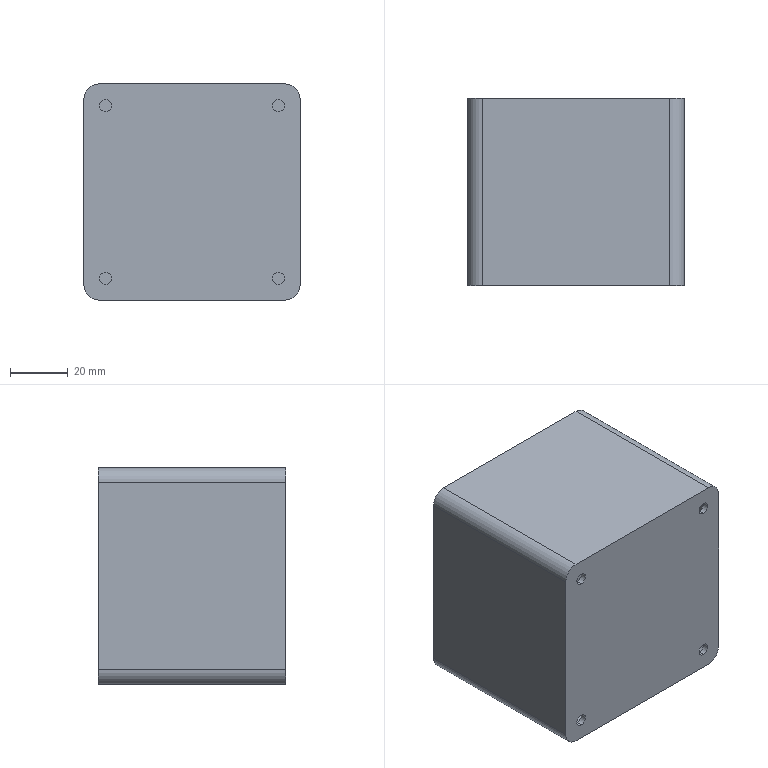Part | STEP file | Guide wheel mechanism revised.sldasm-Part-334 | 1 solid | 30 faces | box 75 x 65 x 75 mm | volume 65636 mm3 | cylinder 18 | plane 12 | commonest cylinder face diameters 4.2 x8 6 x4 10 x4 22 x2
STEP:
#1=CARTESIAN_POINT('',(30.,-30.5,32.1));
#2=VERTEX_POINT('',#1);
#3=CARTESIAN_POINT('',(30.,-30.5,27.9));
#4=VERTEX_POINT('',#3);
#5=CARTESIAN_POINT('',(30.,-30.5,30.));
#6=DIRECTION('',(0.,-1.,0.));
#7=DIRECTION('',(0.,0.,-1.));
#8=AXIS2_PLACEMENT_3D('',#5,#6,#7);
#9=CIRCLE('',#8,2.1);
#10=EDGE_CURVE('',#2,#4,#9,.T.);
#11=ORIENTED_EDGE('',*,*,#10,.F.);
#12=CARTESIAN_POINT('',(30.,-32.5,32.1));
#13=VERTEX_POINT('',#12);
#14=CARTESIAN_POINT('',(30.,-27.5,32.1));
#15=DIRECTION('',(0.,-1.,0.));
#16=VECTOR('',#15,1000.);
#17=LINE('',#14,#16);
#18=EDGE_CURVE('',#2,#13,#17,.T.);
#19=ORIENTED_EDGE('',*,*,#18,.T.);
#20=CARTESIAN_POINT('',(30.,-32.5,27.9));
#21=VERTEX_POINT('',#20);
#22=CARTESIAN_POINT('',(30.,-32.5,30.));
#23=DIRECTION('',(0.,-1.,0.));
#24=DIRECTION('',(0.,0.,1.));
#25=AXIS2_PLACEMENT_3D('',#22,#23,#24);
#26=CIRCLE('',#25,2.1);
#27=EDGE_CURVE('',#13,#21,#26,.T.);
#28=ORIENTED_EDGE('',*,*,#27,.T.);
#29=CARTESIAN_POINT('',(30.,-27.5,27.9));
#30=DIRECTION('',(0.,-1.,0.));
#31=VECTOR('',#30,1000.);
#32=LINE('',#29,#31);
#33=EDGE_CURVE('',#4,#21,#32,.T.);
#34=ORIENTED_EDGE('',*,*,#33,.F.);
#35=EDGE_LOOP('',(#11,#19,#28,#34));
#36=FACE_OUTER_BOUND('',#35,.T.);
#37=CARTESIAN_POINT('',(30.,-27.5,30.));
#38=DIRECTION('',(0.,-1.,0.));
#39=DIRECTION('',(0.,0.,-1.));
#40=AXIS2_PLACEMENT_3D('',#37,#38,#39);
#41=CYLINDRICAL_SURFACE('',#40,2.1);
#42=ADVANCED_FACE('',(#36),#41,.F.);
#43=CARTESIAN_POINT('',(30.,-30.5,-27.9));
#44=VERTEX_POINT('',#43);
#45=CARTESIAN_POINT('',(30.,-30.5,-32.1));
#46=VERTEX_POINT('',#45);
#47=CARTESIAN_POINT('',(30.,-30.5,-30.));
#48=DIRECTION('',(0.,-1.,0.));
#49=DIRECTION('',(0.,0.,-1.));
#50=AXIS2_PLACEMENT_3D('',#47,#48,#49);
#51=CIRCLE('',#50,2.1);
#52=EDGE_CURVE('',#44,#46,#51,.T.);
#53=ORIENTED_EDGE('',*,*,#52,.F.);
#54=CARTESIAN_POINT('',(30.,-32.5,-27.9));
#55=VERTEX_POINT('',#54);
#56=CARTESIAN_POINT('',(30.,-27.5,-27.9));
#57=DIRECTION('',(0.,-1.,0.));
#58=VECTOR('',#57,1000.);
#59=LINE('',#56,#58);
#60=EDGE_CURVE('',#44,#55,#59,.T.);
#61=ORIENTED_EDGE('',*,*,#60,.T.);
#62=CARTESIAN_POINT('',(30.,-32.5,-32.1));
#63=VERTEX_POINT('',#62);
#64=CARTESIAN_POINT('',(30.,-32.5,-30.));
#65=DIRECTION('',(0.,-1.,0.));
#66=DIRECTION('',(0.,0.,-1.));
#67=AXIS2_PLACEMENT_3D('',#64,#65,#66);
#68=CIRCLE('',#67,2.1);
#69=EDGE_CURVE('',#55,#63,#68,.T.);
#70=ORIENTED_EDGE('',*,*,#69,.T.);
#71=CARTESIAN_POINT('',(30.,-27.5,-32.1));
#72=DIRECTION('',(0.,-1.,0.));
#73=VECTOR('',#72,1000.);
#74=LINE('',#71,#73);
#75=EDGE_CURVE('',#46,#63,#74,.T.);
#76=ORIENTED_EDGE('',*,*,#75,.F.);
#77=EDGE_LOOP('',(#53,#61,#70,#76));
#78=FACE_OUTER_BOUND('',#77,.T.);
#79=CARTESIAN_POINT('',(30.,-27.5,-30.));
#80=DIRECTION('',(0.,-1.,0.));
#81=DIRECTION('',(0.,0.,-1.));
#82=AXIS2_PLACEMENT_3D('',#79,#80,#81);
#83=CYLINDRICAL_SURFACE('',#82,2.1);
#84=ADVANCED_FACE('',(#78),#83,.F.);
#85=CARTESIAN_POINT('',(-30.,-30.5,-27.9));
#86=VERTEX_POINT('',#85);
#87=CARTESIAN_POINT('',(-30.,-30.5,-32.1));
#88=VERTEX_POINT('',#87);
#89=CARTESIAN_POINT('',(-30.,-30.5,-30.));
#90=DIRECTION('',(0.,-1.,0.));
#91=DIRECTION('',(0.,0.,-1.));
#92=AXIS2_PLACEMENT_3D('',#89,#90,#91);
#93=CIRCLE('',#92,2.1);
#94=EDGE_CURVE('',#86,#88,#93,.T.);
#95=ORIENTED_EDGE('',*,*,#94,.F.);
#96=CARTESIAN_POINT('',(-30.,-32.5,-27.9));
#97=VERTEX_POINT('',#96);
#98=CARTESIAN_POINT('',(-30.,-27.5,-27.9));
#99=DIRECTION('',(0.,-1.,0.));
#100=VECTOR('',#99,1000.);
#101=LINE('',#98,#100);
#102=EDGE_CURVE('',#86,#97,#101,.T.);
#103=ORIENTED_EDGE('',*,*,#102,.T.);
#104=CARTESIAN_POINT('',(-30.,-32.5,-32.1));
#105=VERTEX_POINT('',#104);
#106=CARTESIAN_POINT('',(-30.,-32.5,-30.));
#107=DIRECTION('',(0.,-1.,0.));
#108=DIRECTION('',(0.,0.,1.));
#109=AXIS2_PLACEMENT_3D('',#106,#107,#108);
#110=CIRCLE('',#109,2.1);
#111=EDGE_CURVE('',#97,#105,#110,.T.);
#112=ORIENTED_EDGE('',*,*,#111,.T.);
#113=CARTESIAN_POINT('',(-30.,-27.5,-32.1));
#114=DIRECTION('',(0.,-1.,0.));
#115=VECTOR('',#114,1000.);
#116=LINE('',#113,#115);
#117=EDGE_CURVE('',#88,#105,#116,.T.);
#118=ORIENTED_EDGE('',*,*,#117,.F.);
#119=EDGE_LOOP('',(#95,#103,#112,#118));
#120=FACE_OUTER_BOUND('',#119,.T.);
#121=CARTESIAN_POINT('',(-30.,-27.5,-30.));
#122=DIRECTION('',(0.,-1.,0.));
#123=DIRECTION('',(0.,0.,-1.));
#124=AXIS2_PLACEMENT_3D('',#121,#122,#123);
#125=CYLINDRICAL_SURFACE('',#124,2.1);
#126=ADVANCED_FACE('',(#120),#125,.F.);
#127=CARTESIAN_POINT('',(-30.,-30.5,32.1));
#128=VERTEX_POINT('',#127);
#129=CARTESIAN_POINT('',(-30.,-30.5,27.9));
#130=VERTEX_POINT('',#129);
#131=CARTESIAN_POINT('',(-30.,-30.5,30.));
#132=DIRECTION('',(0.,-1.,0.));
#133=DIRECTION('',(0.,0.,-1.));
#134=AXIS2_PLACEMENT_3D('',#131,#132,#133);
#135=CIRCLE('',#134,2.1);
#136=EDGE_CURVE('',#128,#130,#135,.T.);
#137=ORIENTED_EDGE('',*,*,#136,.F.);
#138=CARTESIAN_POINT('',(-30.,-32.5,32.1));
#139=VERTEX_POINT('',#138);
#140=CARTESIAN_POINT('',(-30.,-27.5,32.1));
#141=DIRECTION('',(0.,-1.,0.));
#142=VECTOR('',#141,1000.);
#143=LINE('',#140,#142);
#144=EDGE_CURVE('',#128,#139,#143,.T.);
#145=ORIENTED_EDGE('',*,*,#144,.T.);
#146=CARTESIAN_POINT('',(-30.,-32.5,27.9));
#147=VERTEX_POINT('',#146);
#148=CARTESIAN_POINT('',(-30.,-32.5,30.));
#149=DIRECTION('',(0.,-1.,0.));
#150=DIRECTION('',(0.,0.,-1.));
#151=AXIS2_PLACEMENT_3D('',#148,#149,#150);
#152=CIRCLE('',#151,2.1);
#153=EDGE_CURVE('',#139,#147,#152,.T.);
#154=ORIENTED_EDGE('',*,*,#153,.T.);
#155=CARTESIAN_POINT('',(-30.,-27.5,27.9));
#156=DIRECTION('',(0.,-1.,0.));
#157=VECTOR('',#156,1000.);
#158=LINE('',#155,#157);
#159=EDGE_CURVE('',#130,#147,#158,.T.);
#160=ORIENTED_EDGE('',*,*,#159,.F.);
#161=EDGE_LOOP('',(#137,#145,#154,#160));
#162=FACE_OUTER_BOUND('',#161,.T.);
#163=CARTESIAN_POINT('',(-30.,-27.5,30.));
#164=DIRECTION('',(0.,-1.,0.));
#165=DIRECTION('',(0.,0.,-1.));
#166=AXIS2_PLACEMENT_3D('',#163,#164,#165);
#167=CYLINDRICAL_SURFACE('',#166,2.1);
#168=ADVANCED_FACE('',(#162),#167,.F.);
#169=CARTESIAN_POINT('',(0.,28.5,-8.5));
#170=VERTEX_POINT('',#169);
#171=CARTESIAN_POINT('',(0.,28.5,13.5));
#172=VERTEX_POINT('',#171);
#173=CARTESIAN_POINT('',(0.,28.5,2.5));
#174=DIRECTION('',(0.,1.,0.));
#175=DIRECTION('',(0.,0.,1.));
#176=AXIS2_PLACEMENT_3D('',#173,#174,#175);
#177=CIRCLE('',#176,11.);
#178=EDGE_CURVE('',#170,#172,#177,.T.);
#179=ORIENTED_EDGE('',*,*,#178,.F.);
#180=CARTESIAN_POINT('',(0.,32.5,-8.5));
#181=VERTEX_POINT('',#180);
#182=CARTESIAN_POINT('',(0.,27.5,-8.5));
#183=DIRECTION('',(0.,1.,0.));
#184=VECTOR('',#183,1000.);
#185=LINE('',#182,#184);
#186=EDGE_CURVE('',#170,#181,#185,.T.);
#187=ORIENTED_EDGE('',*,*,#186,.T.);
#188=CARTESIAN_POINT('',(0.,32.5,13.5));
#189=VERTEX_POINT('',#188);
#190=CARTESIAN_POINT('',(0.,32.5,2.5));
#191=DIRECTION('',(0.,1.,0.));
#192=DIRECTION('',(0.,0.,1.));
#193=AXIS2_PLACEMENT_3D('',#190,#191,#192);
#194=CIRCLE('',#193,11.);
#195=EDGE_CURVE('',#181,#189,#194,.T.);
#196=ORIENTED_EDGE('',*,*,#195,.T.);
#197=CARTESIAN_POINT('',(0.,27.5,13.5));
#198=DIRECTION('',(0.,1.,0.));
#199=VECTOR('',#198,1000.);
#200=LINE('',#197,#199);
#201=EDGE_CURVE('',#172,#189,#200,.T.);
#202=ORIENTED_EDGE('',*,*,#201,.F.);
#203=EDGE_LOOP('',(#179,#187,#196,#202));
#204=FACE_OUTER_BOUND('',#203,.T.);
#205=CARTESIAN_POINT('',(0.,27.5,2.5));
#206=DIRECTION('',(0.,1.,0.));
#207=DIRECTION('',(0.,0.,1.));
#208=AXIS2_PLACEMENT_3D('',#205,#206,#207);
#209=CYLINDRICAL_SURFACE('',#208,11.);
#210=ADVANCED_FACE('',(#204),#209,.F.);
#211=CARTESIAN_POINT('',(0.,28.5,2.5));
#212=DIRECTION('',(0.,1.,0.));
#213=DIRECTION('',(0.,0.,1.));
#214=AXIS2_PLACEMENT_3D('',#211,#212,#213);
#215=CIRCLE('',#214,11.);
#216=EDGE_CURVE('',#172,#170,#215,.T.);
#217=ORIENTED_EDGE('',*,*,#216,.T.);
#218=ORIENTED_EDGE('',*,*,#178,.T.);
#219=EDGE_LOOP('',(#217,#218));
#220=FACE_BOUND('',#219,.T.);
#221=CARTESIAN_POINT('',(32.5,28.5,-35.5));
#222=VERTEX_POINT('',#221);
#223=CARTESIAN_POINT('',(-32.5,28.5,-35.5));
#224=VERTEX_POINT('',#223);
#225=CARTESIAN_POINT('',(37.5,28.5,-35.5));
#226=DIRECTION('',(-1.,0.,0.));
#227=VECTOR('',#226,1000.);
#228=LINE('',#225,#227);
#229=EDGE_CURVE('',#222,#224,#228,.T.);
#230=ORIENTED_EDGE('',*,*,#229,.F.);
#231=CARTESIAN_POINT('',(35.5,28.5,-32.5));
#232=VERTEX_POINT('',#231);
#233=CARTESIAN_POINT('',(32.5,28.5,-32.5));
#234=DIRECTION('',(0.,-1.,0.));
#235=DIRECTION('',(0.,0.,1.));
#236=AXIS2_PLACEMENT_3D('',#233,#234,#235);
#237=CIRCLE('',#236,3.);
#238=EDGE_CURVE('',#222,#232,#237,.T.);
#239=ORIENTED_EDGE('',*,*,#238,.T.);
#240=CARTESIAN_POINT('',(35.5,28.5,32.5));
#241=VERTEX_POINT('',#240);
#242=CARTESIAN_POINT('',(35.5,28.5,-37.5));
#243=DIRECTION('',(0.,0.,-1.));
#244=VECTOR('',#243,1000.);
#245=LINE('',#242,#244);
#246=EDGE_CURVE('',#241,#232,#245,.T.);
#247=ORIENTED_EDGE('',*,*,#246,.F.);
#248=CARTESIAN_POINT('',(32.5,28.5,35.5));
#249=VERTEX_POINT('',#248);
#250=CARTESIAN_POINT('',(32.5,28.5,32.5));
#251=DIRECTION('',(0.,-1.,0.));
#252=DIRECTION('',(0.,0.,1.));
#253=AXIS2_PLACEMENT_3D('',#250,#251,#252);
#254=CIRCLE('',#253,3.);
#255=EDGE_CURVE('',#241,#249,#254,.T.);
#256=ORIENTED_EDGE('',*,*,#255,.T.);
#257=CARTESIAN_POINT('',(-32.5,28.5,35.5));
#258=VERTEX_POINT('',#257);
#259=CARTESIAN_POINT('',(37.5,28.5,35.5));
#260=DIRECTION('',(1.,0.,0.));
#261=VECTOR('',#260,1000.);
#262=LINE('',#259,#261);
#263=EDGE_CURVE('',#258,#249,#262,.T.);
#264=ORIENTED_EDGE('',*,*,#263,.F.);
#265=CARTESIAN_POINT('',(-35.5,28.5,32.5));
#266=VERTEX_POINT('',#265);
#267=CARTESIAN_POINT('',(-32.5,28.5,32.5));
#268=DIRECTION('',(0.,-1.,0.));
#269=DIRECTION('',(0.,0.,1.));
#270=AXIS2_PLACEMENT_3D('',#267,#268,#269);
#271=CIRCLE('',#270,3.);
#272=EDGE_CURVE('',#258,#266,#271,.T.);
#273=ORIENTED_EDGE('',*,*,#272,.T.);
#274=CARTESIAN_POINT('',(-35.5,28.5,-32.5));
#275=VERTEX_POINT('',#274);
#276=CARTESIAN_POINT('',(-35.5,28.5,-37.5));
#277=DIRECTION('',(0.,0.,1.));
#278=VECTOR('',#277,1000.);
#279=LINE('',#276,#278);
#280=EDGE_CURVE('',#275,#266,#279,.T.);
#281=ORIENTED_EDGE('',*,*,#280,.F.);
#282=CARTESIAN_POINT('',(-32.5,28.5,-32.5));
#283=DIRECTION('',(0.,-1.,0.));
#284=DIRECTION('',(0.,0.,1.));
#285=AXIS2_PLACEMENT_3D('',#282,#283,#284);
#286=CIRCLE('',#285,3.);
#287=EDGE_CURVE('',#275,#224,#286,.T.);
#288=ORIENTED_EDGE('',*,*,#287,.T.);
#289=EDGE_LOOP('',(#230,#239,#247,#256,#264,#273,#281,#288));
#290=FACE_OUTER_BOUND('',#289,.T.);
#291=CARTESIAN_POINT('',(32.5,28.5,32.5));
#292=DIRECTION('',(0.,1.,0.));
#293=DIRECTION('',(0.,0.,1.));
#294=AXIS2_PLACEMENT_3D('',#291,#292,#293);
#295=PLANE('',#294);
#296=ADVANCED_FACE('',(#220,#290),#295,.F.);
#297=CARTESIAN_POINT('',(30.,-30.5,30.));
#298=DIRECTION('',(0.,-1.,0.));
#299=DIRECTION('',(0.,0.,-1.));
#300=AXIS2_PLACEMENT_3D('',#297,#298,#299);
#301=CIRCLE('',#300,2.1);
#302=EDGE_CURVE('',#4,#2,#301,.T.);
#303=ORIENTED_EDGE('',*,*,#302,.T.);
#304=ORIENTED_EDGE('',*,*,#10,.T.);
#305=EDGE_LOOP('',(#303,#304));
#306=FACE_BOUND('',#305,.T.);
#307=CARTESIAN_POINT('',(30.,-30.5,-30.));
#308=DIRECTION('',(0.,-1.,0.));
#309=DIRECTION('',(0.,0.,-1.));
#310=AXIS2_PLACEMENT_3D('',#307,#308,#309);
#311=CIRCLE('',#310,2.1);
#312=EDGE_CURVE('',#46,#44,#311,.T.);
#313=ORIENTED_EDGE('',*,*,#312,.T.);
#314=ORIENTED_EDGE('',*,*,#52,.T.);
#315=EDGE_LOOP('',(#313,#314));
#316=FACE_BOUND('',#315,.T.);
#317=CARTESIAN_POINT('',(-30.,-30.5,-30.));
#318=DIRECTION('',(0.,-1.,0.));
#319=DIRECTION('',(0.,0.,-1.));
#320=AXIS2_PLACEMENT_3D('',#317,#318,#319);
#321=CIRCLE('',#320,2.1);
#322=EDGE_CURVE('',#88,#86,#321,.T.);
#323=ORIENTED_EDGE('',*,*,#322,.T.);
#324=ORIENTED_EDGE('',*,*,#94,.T.);
#325=EDGE_LOOP('',(#323,#324));
#326=FACE_BOUND('',#325,.T.);
#327=CARTESIAN_POINT('',(-30.,-30.5,30.));
#328=DIRECTION('',(0.,-1.,0.));
#329=DIRECTION('',(0.,0.,-1.));
#330=AXIS2_PLACEMENT_3D('',#327,#328,#329);
#331=CIRCLE('',#330,2.1);
#332=EDGE_CURVE('',#130,#128,#331,.T.);
#333=ORIENTED_EDGE('',*,*,#332,.T.);
#334=ORIENTED_EDGE('',*,*,#136,.T.);
#335=EDGE_LOOP('',(#333,#334));
#336=FACE_BOUND('',#335,.T.);
#337=CARTESIAN_POINT('',(32.5,-30.5,-35.5));
#338=VERTEX_POINT('',#337);
#339=CARTESIAN_POINT('',(-32.5,-30.5,-35.5));
#340=VERTEX_POINT('',#339);
#341=CARTESIAN_POINT('',(-37.5,-30.5,-35.5));
#342=DIRECTION('',(-1.,0.,0.));
#343=VECTOR('',#342,1000.);
#344=LINE('',#341,#343);
#345=EDGE_CURVE('',#338,#340,#344,.T.);
#346=ORIENTED_EDGE('',*,*,#345,.T.);
#347=CARTESIAN_POINT('',(-35.5,-30.5,-32.5));
#348=VERTEX_POINT('',#347);
#349=CARTESIAN_POINT('',(-32.5,-30.5,-32.5));
#350=DIRECTION('',(0.,-1.,0.));
#351=DIRECTION('',(0.,0.,-1.));
#352=AXIS2_PLACEMENT_3D('',#349,#350,#351);
#353=CIRCLE('',#352,3.);
#354=EDGE_CURVE('',#348,#340,#353,.T.);
#355=ORIENTED_EDGE('',*,*,#354,.F.);
#356=CARTESIAN_POINT('',(-35.5,-30.5,32.5));
#357=VERTEX_POINT('',#356);
#358=CARTESIAN_POINT('',(-35.5,-30.5,37.5));
#359=DIRECTION('',(0.,0.,1.));
#360=VECTOR('',#359,1000.);
#361=LINE('',#358,#360);
#362=EDGE_CURVE('',#348,#357,#361,.T.);
#363=ORIENTED_EDGE('',*,*,#362,.T.);
#364=CARTESIAN_POINT('',(-32.5,-30.5,35.5));
#365=VERTEX_POINT('',#364);
#366=CARTESIAN_POINT('',(-32.5,-30.5,32.5));
#367=DIRECTION('',(0.,-1.,0.));
#368=DIRECTION('',(0.,0.,-1.));
#369=AXIS2_PLACEMENT_3D('',#366,#367,#368);
#370=CIRCLE('',#369,3.);
#371=EDGE_CURVE('',#365,#357,#370,.T.);
#372=ORIENTED_EDGE('',*,*,#371,.F.);
#373=CARTESIAN_POINT('',(32.5,-30.5,35.5));
#374=VERTEX_POINT('',#373);
#375=CARTESIAN_POINT('',(-37.5,-30.5,35.5));
#376=DIRECTION('',(1.,0.,0.));
#377=VECTOR('',#376,1000.);
#378=LINE('',#375,#377);
#379=EDGE_CURVE('',#365,#374,#378,.T.);
#380=ORIENTED_EDGE('',*,*,#379,.T.);
#381=CARTESIAN_POINT('',(35.5,-30.5,32.5));
#382=VERTEX_POINT('',#381);
#383=CARTESIAN_POINT('',(32.5,-30.5,32.5));
#384=DIRECTION('',(0.,-1.,0.));
#385=DIRECTION('',(0.,0.,-1.));
#386=AXIS2_PLACEMENT_3D('',#383,#384,#385);
#387=CIRCLE('',#386,3.);
#388=EDGE_CURVE('',#382,#374,#387,.T.);
#389=ORIENTED_EDGE('',*,*,#388,.F.);
#390=CARTESIAN_POINT('',(35.5,-30.5,-32.5));
#391=VERTEX_POINT('',#390);
#392=CARTESIAN_POINT('',(35.5,-30.5,37.5));
#393=DIRECTION('',(0.,0.,-1.));
#394=VECTOR('',#393,1000.);
#395=LINE('',#392,#394);
#396=EDGE_CURVE('',#382,#391,#395,.T.);
#397=ORIENTED_EDGE('',*,*,#396,.T.);
#398=CARTESIAN_POINT('',(32.5,-30.5,-32.5));
#399=DIRECTION('',(0.,-1.,0.));
#400=DIRECTION('',(0.,0.,-1.));
#401=AXIS2_PLACEMENT_3D('',#398,#399,#400);
#402=CIRCLE('',#401,3.);
#403=EDGE_CURVE('',#338,#391,#402,.T.);
#404=ORIENTED_EDGE('',*,*,#403,.F.);
#405=EDGE_LOOP('',(#346,#355,#363,#372,#380,#389,#397,#404));
#406=FACE_OUTER_BOUND('',#405,.T.);
#407=CARTESIAN_POINT('',(-37.5,-30.5,37.5));
#408=DIRECTION('',(0.,-1.,0.));
#409=DIRECTION('',(0.,0.,-1.));
#410=AXIS2_PLACEMENT_3D('',#407,#408,#409);
#411=PLANE('',#410);
#412=ADVANCED_FACE('',(#306,#316,#326,#336,#406),#411,.F.);
#413=ORIENTED_EDGE('',*,*,#287,.F.);
#414=CARTESIAN_POINT('',(-35.5,32.5,-32.5));
#415=DIRECTION('',(0.,-1.,0.));
#416=VECTOR('',#415,1000.);
#417=LINE('',#414,#416);
#418=EDGE_CURVE('',#275,#348,#417,.T.);
#419=ORIENTED_EDGE('',*,*,#418,.T.);
#420=ORIENTED_EDGE('',*,*,#354,.T.);
#421=CARTESIAN_POINT('',(-32.5,32.5,-35.5));
#422=DIRECTION('',(0.,1.,0.));
#423=VECTOR('',#422,1000.);
#424=LINE('',#421,#423);
#425=EDGE_CURVE('',#340,#224,#424,.T.);
#426=ORIENTED_EDGE('',*,*,#425,.T.);
#427=EDGE_LOOP('',(#413,#419,#420,#426));
#428=FACE_OUTER_BOUND('',#427,.T.);
#429=CARTESIAN_POINT('',(-32.5,32.5,-32.5));
#430=DIRECTION('',(0.,-1.,0.));
#431=DIRECTION('',(0.,0.,-1.));
#432=AXIS2_PLACEMENT_3D('',#429,#430,#431);
#433=CYLINDRICAL_SURFACE('',#432,3.);
#434=ADVANCED_FACE('',(#428),#433,.F.);
#435=ORIENTED_EDGE('',*,*,#238,.F.);
#436=CARTESIAN_POINT('',(32.5,32.5,-35.5));
#437=DIRECTION('',(0.,-1.,0.));
#438=VECTOR('',#437,1000.);
#439=LINE('',#436,#438);
#440=EDGE_CURVE('',#222,#338,#439,.T.);
#441=ORIENTED_EDGE('',*,*,#440,.T.);
#442=ORIENTED_EDGE('',*,*,#403,.T.);
#443=CARTESIAN_POINT('',(35.5,32.5,-32.5));
#444=DIRECTION('',(0.,1.,0.));
#445=VECTOR('',#444,1000.);
#446=LINE('',#443,#445);
#447=EDGE_CURVE('',#391,#232,#446,.T.);
#448=ORIENTED_EDGE('',*,*,#447,.T.);
#449=EDGE_LOOP('',(#435,#441,#442,#448));
#450=FACE_OUTER_BOUND('',#449,.T.);
#451=CARTESIAN_POINT('',(32.5,32.5,-32.5));
#452=DIRECTION('',(0.,-1.,0.));
#453=DIRECTION('',(0.,0.,-1.));
#454=AXIS2_PLACEMENT_3D('',#451,#452,#453);
#455=CYLINDRICAL_SURFACE('',#454,3.);
#456=ADVANCED_FACE('',(#450),#455,.F.);
#457=ORIENTED_EDGE('',*,*,#440,.F.);
#458=ORIENTED_EDGE('',*,*,#229,.T.);
#459=ORIENTED_EDGE('',*,*,#425,.F.);
#460=ORIENTED_EDGE('',*,*,#345,.F.);
#461=EDGE_LOOP('',(#457,#458,#459,#460));
#462=FACE_OUTER_BOUND('',#461,.T.);
#463=CARTESIAN_POINT('',(37.5,32.5,-35.5));
#464=DIRECTION('',(0.,0.,1.));
#465=DIRECTION('',(1.,0.,0.));
#466=AXIS2_PLACEMENT_3D('',#463,#464,#465);
#467=PLANE('',#466);
#468=ADVANCED_FACE('',(#462),#467,.T.);
#469=ORIENTED_EDGE('',*,*,#255,.F.);
#470=CARTESIAN_POINT('',(35.5,32.5,32.5));
#471=DIRECTION('',(0.,-1.,0.));
#472=VECTOR('',#471,1000.);
#473=LINE('',#470,#472);
#474=EDGE_CURVE('',#241,#382,#473,.T.);
#475=ORIENTED_EDGE('',*,*,#474,.T.);
#476=ORIENTED_EDGE('',*,*,#388,.T.);
#477=CARTESIAN_POINT('',(32.5,32.5,35.5));
#478=DIRECTION('',(0.,1.,0.));
#479=VECTOR('',#478,1000.);
#480=LINE('',#477,#479);
#481=EDGE_CURVE('',#374,#249,#480,.T.);
#482=ORIENTED_EDGE('',*,*,#481,.T.);
#483=EDGE_LOOP('',(#469,#475,#476,#482));
#484=FACE_OUTER_BOUND('',#483,.T.);
#485=CARTESIAN_POINT('',(32.5,32.5,32.5));
#486=DIRECTION('',(0.,-1.,0.));
#487=DIRECTION('',(0.,0.,-1.));
#488=AXIS2_PLACEMENT_3D('',#485,#486,#487);
#489=CYLINDRICAL_SURFACE('',#488,3.);
#490=ADVANCED_FACE('',(#484),#489,.F.);
#491=ORIENTED_EDGE('',*,*,#474,.F.);
#492=ORIENTED_EDGE('',*,*,#246,.T.);
#493=ORIENTED_EDGE('',*,*,#447,.F.);
#494=ORIENTED_EDGE('',*,*,#396,.F.);
#495=EDGE_LOOP('',(#491,#492,#493,#494));
#496=FACE_OUTER_BOUND('',#495,.T.);
#497=CARTESIAN_POINT('',(35.5,32.5,-37.5));
#498=DIRECTION('',(-1.,0.,0.));
#499=DIRECTION('',(0.,0.,1.));
#500=AXIS2_PLACEMENT_3D('',#497,#498,#499);
#501=PLANE('',#500);
#502=ADVANCED_FACE('',(#496),#501,.T.);
#503=ORIENTED_EDGE('',*,*,#272,.F.);
#504=CARTESIAN_POINT('',(-32.5,32.5,35.5));
#505=DIRECTION('',(0.,-1.,0.));
#506=VECTOR('',#505,1000.);
#507=LINE('',#504,#506);
#508=EDGE_CURVE('',#258,#365,#507,.T.);
#509=ORIENTED_EDGE('',*,*,#508,.T.);
#510=ORIENTED_EDGE('',*,*,#371,.T.);
#511=CARTESIAN_POINT('',(-35.5,32.5,32.5));
#512=DIRECTION('',(0.,1.,0.));
#513=VECTOR('',#512,1000.);
#514=LINE('',#511,#513);
#515=EDGE_CURVE('',#357,#266,#514,.T.);
#516=ORIENTED_EDGE('',*,*,#515,.T.);
#517=EDGE_LOOP('',(#503,#509,#510,#516));
#518=FACE_OUTER_BOUND('',#517,.T.);
#519=CARTESIAN_POINT('',(-32.5,32.5,32.5));
#520=DIRECTION('',(0.,-1.,0.));
#521=DIRECTION('',(0.,0.,-1.));
#522=AXIS2_PLACEMENT_3D('',#519,#520,#521);
#523=CYLINDRICAL_SURFACE('',#522,3.);
#524=ADVANCED_FACE('',(#518),#523,.F.);
#525=ORIENTED_EDGE('',*,*,#508,.F.);
#526=ORIENTED_EDGE('',*,*,#263,.T.);
#527=ORIENTED_EDGE('',*,*,#481,.F.);
#528=ORIENTED_EDGE('',*,*,#379,.F.);
#529=EDGE_LOOP('',(#525,#526,#527,#528));
#530=FACE_OUTER_BOUND('',#529,.T.);
#531=CARTESIAN_POINT('',(37.5,32.5,35.5));
#532=DIRECTION('',(0.,0.,-1.));
#533=DIRECTION('',(-1.,0.,0.));
#534=AXIS2_PLACEMENT_3D('',#531,#532,#533);
#535=PLANE('',#534);
#536=ADVANCED_FACE('',(#530),#535,.T.);
#537=ORIENTED_EDGE('',*,*,#418,.F.);
#538=ORIENTED_EDGE('',*,*,#280,.T.);
#539=ORIENTED_EDGE('',*,*,#515,.F.);
#540=ORIENTED_EDGE('',*,*,#362,.F.);
#541=EDGE_LOOP('',(#537,#538,#539,#540));
#542=FACE_OUTER_BOUND('',#541,.T.);
#543=CARTESIAN_POINT('',(-35.5,32.5,-37.5));
#544=DIRECTION('',(1.,0.,0.));
#545=DIRECTION('',(0.,0.,-1.));
#546=AXIS2_PLACEMENT_3D('',#543,#544,#545);
#547=PLANE('',#546);
#548=ADVANCED_FACE('',(#542),#547,.T.);
#549=ORIENTED_EDGE('',*,*,#186,.F.);
#550=ORIENTED_EDGE('',*,*,#216,.F.);
#551=ORIENTED_EDGE('',*,*,#201,.T.);
#552=CARTESIAN_POINT('',(0.,32.5,2.5));
#553=DIRECTION('',(0.,1.,0.));
#554=DIRECTION('',(0.,0.,1.));
#555=AXIS2_PLACEMENT_3D('',#552,#553,#554);
#556=CIRCLE('',#555,11.);
#557=EDGE_CURVE('',#189,#181,#556,.T.);
#558=ORIENTED_EDGE('',*,*,#557,.T.);
#559=EDGE_LOOP('',(#549,#550,#551,#558));
#560=FACE_OUTER_BOUND('',#559,.T.);
#561=CARTESIAN_POINT('',(0.,27.5,2.5));
#562=DIRECTION('',(0.,1.,0.));
#563=DIRECTION('',(0.,0.,1.));
#564=AXIS2_PLACEMENT_3D('',#561,#562,#563);
#565=CYLINDRICAL_SURFACE('',#564,11.);
#566=ADVANCED_FACE('',(#560),#565,.F.);
#567=ORIENTED_EDGE('',*,*,#557,.F.);
#568=ORIENTED_EDGE('',*,*,#195,.F.);
#569=EDGE_LOOP('',(#567,#568));
#570=FACE_BOUND('',#569,.T.);
#571=CARTESIAN_POINT('',(37.5,32.5,32.5));
#572=VERTEX_POINT('',#571);
#573=CARTESIAN_POINT('',(37.5,32.5,-32.5));
#574=VERTEX_POINT('',#573);
#575=CARTESIAN_POINT('',(37.5,32.5,-37.5));
#576=DIRECTION('',(0.,0.,-1.));
#577=VECTOR('',#576,1000.);
#578=LINE('',#575,#577);
#579=EDGE_CURVE('',#572,#574,#578,.T.);
#580=ORIENTED_EDGE('',*,*,#579,.T.);
#581=CARTESIAN_POINT('',(32.5,32.5,-37.5));
#582=VERTEX_POINT('',#581);
#583=CARTESIAN_POINT('',(32.5,32.5,-32.5));
#584=DIRECTION('',(0.,1.,0.));
#585=DIRECTION('',(0.,0.,-1.));
#586=AXIS2_PLACEMENT_3D('',#583,#584,#585);
#587=CIRCLE('',#586,5.);
#588=EDGE_CURVE('',#574,#582,#587,.T.);
#589=ORIENTED_EDGE('',*,*,#588,.T.);
#590=CARTESIAN_POINT('',(-32.5,32.5,-37.5));
#591=VERTEX_POINT('',#590);
#592=CARTESIAN_POINT('',(37.5,32.5,-37.5));
#593=DIRECTION('',(-1.,0.,0.));
#594=VECTOR('',#593,1000.);
#595=LINE('',#592,#594);
#596=EDGE_CURVE('',#582,#591,#595,.T.);
#597=ORIENTED_EDGE('',*,*,#596,.T.);
#598=CARTESIAN_POINT('',(-37.5,32.5,-32.5));
#599=VERTEX_POINT('',#598);
#600=CARTESIAN_POINT('',(-32.5,32.5,-32.5));
#601=DIRECTION('',(0.,1.,0.));
#602=DIRECTION('',(0.,0.,-1.));
#603=AXIS2_PLACEMENT_3D('',#600,#601,#602);
#604=CIRCLE('',#603,5.);
#605=EDGE_CURVE('',#591,#599,#604,.T.);
#606=ORIENTED_EDGE('',*,*,#605,.T.);
#607=CARTESIAN_POINT('',(-37.5,32.5,32.5));
#608=VERTEX_POINT('',#607);
#609=CARTESIAN_POINT('',(-37.5,32.5,-37.5));
#610=DIRECTION('',(0.,0.,1.));
#611=VECTOR('',#610,1000.);
#612=LINE('',#609,#611);
#613=EDGE_CURVE('',#599,#608,#612,.T.);
#614=ORIENTED_EDGE('',*,*,#613,.T.);
#615=CARTESIAN_POINT('',(-32.5,32.5,37.5));
#616=VERTEX_POINT('',#615);
#617=CARTESIAN_POINT('',(-32.5,32.5,32.5));
#618=DIRECTION('',(0.,1.,0.));
#619=DIRECTION('',(0.,0.,-1.));
#620=AXIS2_PLACEMENT_3D('',#617,#618,#619);
#621=CIRCLE('',#620,5.);
#622=EDGE_CURVE('',#608,#616,#621,.T.);
#623=ORIENTED_EDGE('',*,*,#622,.T.);
#624=CARTESIAN_POINT('',(32.5,32.5,37.5));
#625=VERTEX_POINT('',#624);
#626=CARTESIAN_POINT('',(37.5,32.5,37.5));
#627=DIRECTION('',(1.,0.,0.));
#628=VECTOR('',#627,1000.);
#629=LINE('',#626,#628);
#630=EDGE_CURVE('',#616,#625,#629,.T.);
#631=ORIENTED_EDGE('',*,*,#630,.T.);
#632=CARTESIAN_POINT('',(32.5,32.5,32.5));
#633=DIRECTION('',(0.,1.,0.));
#634=DIRECTION('',(0.,0.,-1.));
#635=AXIS2_PLACEMENT_3D('',#632,#633,#634);
#636=CIRCLE('',#635,5.);
#637=EDGE_CURVE('',#625,#572,#636,.T.);
#638=ORIENTED_EDGE('',*,*,#637,.T.);
#639=EDGE_LOOP('',(#580,#589,#597,#606,#614,#623,#631,#638));
#640=FACE_OUTER_BOUND('',#639,.T.);
#641=CARTESIAN_POINT('',(-37.5,32.5,37.5));
#642=DIRECTION('',(0.,-1.,0.));
#643=DIRECTION('',(0.,0.,-1.));
#644=AXIS2_PLACEMENT_3D('',#641,#642,#643);
#645=PLANE('',#644);
#646=ADVANCED_FACE('',(#570,#640),#645,.F.);
#647=CARTESIAN_POINT('',(-37.5,-32.5,-32.5));
#648=VERTEX_POINT('',#647);
#649=CARTESIAN_POINT('',(-37.5,32.5,-32.5));
#650=DIRECTION('',(0.,-1.,0.));
#651=VECTOR('',#650,1000.);
#652=LINE('',#649,#651);
#653=EDGE_CURVE('',#599,#648,#652,.T.);
#654=ORIENTED_EDGE('',*,*,#653,.T.);
#655=CARTESIAN_POINT('',(-37.5,-32.5,32.5));
#656=VERTEX_POINT('',#655);
#657=CARTESIAN_POINT('',(-37.5,-32.5,-37.5));
#658=DIRECTION('',(0.,0.,1.));
#659=VECTOR('',#658,1000.);
#660=LINE('',#657,#659);
#661=EDGE_CURVE('',#648,#656,#660,.T.);
#662=ORIENTED_EDGE('',*,*,#661,.T.);
#663=CARTESIAN_POINT('',(-37.5,32.5,32.5));
#664=DIRECTION('',(0.,1.,0.));
#665=VECTOR('',#664,1000.);
#666=LINE('',#663,#665);
#667=EDGE_CURVE('',#656,#608,#666,.T.);
#668=ORIENTED_EDGE('',*,*,#667,.T.);
#669=ORIENTED_EDGE('',*,*,#613,.F.);
#670=EDGE_LOOP('',(#654,#662,#668,#669));
#671=FACE_OUTER_BOUND('',#670,.T.);
#672=CARTESIAN_POINT('',(-37.5,32.5,-37.5));
#673=DIRECTION('',(1.,0.,0.));
#674=DIRECTION('',(0.,0.,-1.));
#675=AXIS2_PLACEMENT_3D('',#672,#673,#674);
#676=PLANE('',#675);
#677=ADVANCED_FACE('',(#671),#676,.F.);
#678=CARTESIAN_POINT('',(-32.5,-32.5,37.5));
#679=VERTEX_POINT('',#678);
#680=CARTESIAN_POINT('',(-32.5,32.5,37.5));
#681=DIRECTION('',(0.,-1.,0.));
#682=VECTOR('',#681,1000.);
#683=LINE('',#680,#682);
#684=EDGE_CURVE('',#616,#679,#683,.T.);
#685=ORIENTED_EDGE('',*,*,#684,.T.);
#686=CARTESIAN_POINT('',(32.5,-32.5,37.5));
#687=VERTEX_POINT('',#686);
#688=CARTESIAN_POINT('',(37.5,-32.5,37.5));
#689=DIRECTION('',(1.,0.,0.));
#690=VECTOR('',#689,1000.);
#691=LINE('',#688,#690);
#692=EDGE_CURVE('',#679,#687,#691,.T.);
#693=ORIENTED_EDGE('',*,*,#692,.T.);
#694=CARTESIAN_POINT('',(32.5,32.5,37.5));
#695=DIRECTION('',(0.,1.,0.));
#696=VECTOR('',#695,1000.);
#697=LINE('',#694,#696);
#698=EDGE_CURVE('',#687,#625,#697,.T.);
#699=ORIENTED_EDGE('',*,*,#698,.T.);
#700=ORIENTED_EDGE('',*,*,#630,.F.);
#701=EDGE_LOOP('',(#685,#693,#699,#700));
#702=FACE_OUTER_BOUND('',#701,.T.);
#703=CARTESIAN_POINT('',(37.5,32.5,37.5));
#704=DIRECTION('',(0.,0.,-1.));
#705=DIRECTION('',(-1.,0.,0.));
#706=AXIS2_PLACEMENT_3D('',#703,#704,#705);
#707=PLANE('',#706);
#708=ADVANCED_FACE('',(#702),#707,.F.);
#709=CARTESIAN_POINT('',(37.5,-32.5,32.5));
#710=VERTEX_POINT('',#709);
#711=CARTESIAN_POINT('',(37.5,32.5,32.5));
#712=DIRECTION('',(0.,-1.,0.));
#713=VECTOR('',#712,1000.);
#714=LINE('',#711,#713);
#715=EDGE_CURVE('',#572,#710,#714,.T.);
#716=ORIENTED_EDGE('',*,*,#715,.T.);
#717=CARTESIAN_POINT('',(37.5,-32.5,-32.5));
#718=VERTEX_POINT('',#717);
#719=CARTESIAN_POINT('',(37.5,-32.5,-37.5));
#720=DIRECTION('',(0.,0.,-1.));
#721=VECTOR('',#720,1000.);
#722=LINE('',#719,#721);
#723=EDGE_CURVE('',#710,#718,#722,.T.);
#724=ORIENTED_EDGE('',*,*,#723,.T.);
#725=CARTESIAN_POINT('',(37.5,32.5,-32.5));
#726=DIRECTION('',(0.,1.,0.));
#727=VECTOR('',#726,1000.);
#728=LINE('',#725,#727);
#729=EDGE_CURVE('',#718,#574,#728,.T.);
#730=ORIENTED_EDGE('',*,*,#729,.T.);
#731=ORIENTED_EDGE('',*,*,#579,.F.);
#732=EDGE_LOOP('',(#716,#724,#730,#731));
#733=FACE_OUTER_BOUND('',#732,.T.);
#734=CARTESIAN_POINT('',(37.5,32.5,-37.5));
#735=DIRECTION('',(-1.,0.,0.));
#736=DIRECTION('',(0.,0.,1.));
#737=AXIS2_PLACEMENT_3D('',#734,#735,#736);
#738=PLANE('',#737);
#739=ADVANCED_FACE('',(#733),#738,.F.);
#740=CARTESIAN_POINT('',(32.5,-32.5,-37.5));
#741=VERTEX_POINT('',#740);
#742=CARTESIAN_POINT('',(32.5,32.5,-37.5));
#743=DIRECTION('',(0.,-1.,0.));
#744=VECTOR('',#743,1000.);
#745=LINE('',#742,#744);
#746=EDGE_CURVE('',#582,#741,#745,.T.);
#747=ORIENTED_EDGE('',*,*,#746,.T.);
#748=CARTESIAN_POINT('',(-32.5,-32.5,-37.5));
#749=VERTEX_POINT('',#748);
#750=CARTESIAN_POINT('',(37.5,-32.5,-37.5));
#751=DIRECTION('',(-1.,0.,0.));
#752=VECTOR('',#751,1000.);
#753=LINE('',#750,#752);
#754=EDGE_CURVE('',#741,#749,#753,.T.);
#755=ORIENTED_EDGE('',*,*,#754,.T.);
#756=CARTESIAN_POINT('',(-32.5,32.5,-37.5));
#757=DIRECTION('',(0.,1.,0.));
#758=VECTOR('',#757,1000.);
#759=LINE('',#756,#758);
#760=EDGE_CURVE('',#749,#591,#759,.T.);
#761=ORIENTED_EDGE('',*,*,#760,.T.);
#762=ORIENTED_EDGE('',*,*,#596,.F.);
#763=EDGE_LOOP('',(#747,#755,#761,#762));
#764=FACE_OUTER_BOUND('',#763,.T.);
#765=CARTESIAN_POINT('',(37.5,32.5,-37.5));
#766=DIRECTION('',(0.,0.,1.));
#767=DIRECTION('',(1.,0.,0.));
#768=AXIS2_PLACEMENT_3D('',#765,#766,#767);
#769=PLANE('',#768);
#770=ADVANCED_FACE('',(#764),#769,.F.);
#771=CARTESIAN_POINT('',(30.,-32.5,30.));
#772=DIRECTION('',(0.,-1.,0.));
#773=DIRECTION('',(0.,0.,1.));
#774=AXIS2_PLACEMENT_3D('',#771,#772,#773);
#775=CIRCLE('',#774,2.1);
#776=EDGE_CURVE('',#21,#13,#775,.T.);
#777=ORIENTED_EDGE('',*,*,#776,.F.);
#778=ORIENTED_EDGE('',*,*,#27,.F.);
#779=EDGE_LOOP('',(#777,#778));
#780=FACE_BOUND('',#779,.T.);
#781=CARTESIAN_POINT('',(30.,-32.5,-30.));
#782=DIRECTION('',(0.,-1.,0.));
#783=DIRECTION('',(0.,0.,-1.));
#784=AXIS2_PLACEMENT_3D('',#781,#782,#783);
#785=CIRCLE('',#784,2.1);
#786=EDGE_CURVE('',#63,#55,#785,.T.);
#787=ORIENTED_EDGE('',*,*,#786,.F.);
#788=ORIENTED_EDGE('',*,*,#69,.F.);
#789=EDGE_LOOP('',(#787,#788));
#790=FACE_BOUND('',#789,.T.);
#791=CARTESIAN_POINT('',(-30.,-32.5,-30.));
#792=DIRECTION('',(0.,-1.,0.));
#793=DIRECTION('',(0.,0.,1.));
#794=AXIS2_PLACEMENT_3D('',#791,#792,#793);
#795=CIRCLE('',#794,2.1);
#796=EDGE_CURVE('',#105,#97,#795,.T.);
#797=ORIENTED_EDGE('',*,*,#796,.F.);
#798=ORIENTED_EDGE('',*,*,#111,.F.);
#799=EDGE_LOOP('',(#797,#798));
#800=FACE_BOUND('',#799,.T.);
#801=CARTESIAN_POINT('',(-30.,-32.5,30.));
#802=DIRECTION('',(0.,-1.,0.));
#803=DIRECTION('',(0.,0.,-1.));
#804=AXIS2_PLACEMENT_3D('',#801,#802,#803);
#805=CIRCLE('',#804,2.1);
#806=EDGE_CURVE('',#147,#139,#805,.T.);
#807=ORIENTED_EDGE('',*,*,#806,.F.);
#808=ORIENTED_EDGE('',*,*,#153,.F.);
#809=EDGE_LOOP('',(#807,#808));
#810=FACE_BOUND('',#809,.T.);
#811=ORIENTED_EDGE('',*,*,#754,.F.);
#812=CARTESIAN_POINT('',(32.5,-32.5,-32.5));
#813=DIRECTION('',(0.,-1.,0.));
#814=DIRECTION('',(0.,0.,-1.));
#815=AXIS2_PLACEMENT_3D('',#812,#813,#814);
#816=CIRCLE('',#815,5.);
#817=EDGE_CURVE('',#741,#718,#816,.T.);
#818=ORIENTED_EDGE('',*,*,#817,.T.);
#819=ORIENTED_EDGE('',*,*,#723,.F.);
#820=CARTESIAN_POINT('',(32.5,-32.5,32.5));
#821=DIRECTION('',(0.,-1.,0.));
#822=DIRECTION('',(0.,0.,-1.));
#823=AXIS2_PLACEMENT_3D('',#820,#821,#822);
#824=CIRCLE('',#823,5.);
#825=EDGE_CURVE('',#710,#687,#824,.T.);
#826=ORIENTED_EDGE('',*,*,#825,.T.);
#827=ORIENTED_EDGE('',*,*,#692,.F.);
#828=CARTESIAN_POINT('',(-32.5,-32.5,32.5));
#829=DIRECTION('',(0.,-1.,0.));
#830=DIRECTION('',(0.,0.,-1.));
#831=AXIS2_PLACEMENT_3D('',#828,#829,#830);
#832=CIRCLE('',#831,5.);
#833=EDGE_CURVE('',#679,#656,#832,.T.);
#834=ORIENTED_EDGE('',*,*,#833,.T.);
#835=ORIENTED_EDGE('',*,*,#661,.F.);
#836=CARTESIAN_POINT('',(-32.5,-32.5,-32.5));
#837=DIRECTION('',(0.,-1.,0.));
#838=DIRECTION('',(0.,0.,-1.));
#839=AXIS2_PLACEMENT_3D('',#836,#837,#838);
#840=CIRCLE('',#839,5.);
#841=EDGE_CURVE('',#648,#749,#840,.T.);
#842=ORIENTED_EDGE('',*,*,#841,.T.);
#843=EDGE_LOOP('',(#811,#818,#819,#826,#827,#834,#835,#842));
#844=FACE_OUTER_BOUND('',#843,.T.);
#845=CARTESIAN_POINT('',(-37.5,-32.5,37.5));
#846=DIRECTION('',(0.,-1.,0.));
#847=DIRECTION('',(0.,0.,-1.));
#848=AXIS2_PLACEMENT_3D('',#845,#846,#847);
#849=PLANE('',#848);
#850=ADVANCED_FACE('',(#780,#790,#800,#810,#844),#849,.T.);
#851=ORIENTED_EDGE('',*,*,#588,.F.);
#852=ORIENTED_EDGE('',*,*,#729,.F.);
#853=ORIENTED_EDGE('',*,*,#817,.F.);
#854=ORIENTED_EDGE('',*,*,#746,.F.);
#855=EDGE_LOOP('',(#851,#852,#853,#854));
#856=FACE_OUTER_BOUND('',#855,.T.);
#857=CARTESIAN_POINT('',(32.5,32.5,-32.5));
#858=DIRECTION('',(0.,-1.,0.));
#859=DIRECTION('',(0.,0.,-1.));
#860=AXIS2_PLACEMENT_3D('',#857,#858,#859);
#861=CYLINDRICAL_SURFACE('',#860,5.);
#862=ADVANCED_FACE('',(#856),#861,.T.);
#863=ORIENTED_EDGE('',*,*,#605,.F.);
#864=ORIENTED_EDGE('',*,*,#760,.F.);
#865=ORIENTED_EDGE('',*,*,#841,.F.);
#866=ORIENTED_EDGE('',*,*,#653,.F.);
#867=EDGE_LOOP('',(#863,#864,#865,#866));
#868=FACE_OUTER_BOUND('',#867,.T.);
#869=CARTESIAN_POINT('',(-32.5,32.5,-32.5));
#870=DIRECTION('',(0.,-1.,0.));
#871=DIRECTION('',(0.,0.,-1.));
#872=AXIS2_PLACEMENT_3D('',#869,#870,#871);
#873=CYLINDRICAL_SURFACE('',#872,5.);
#874=ADVANCED_FACE('',(#868),#873,.T.);
#875=ORIENTED_EDGE('',*,*,#637,.F.);
#876=ORIENTED_EDGE('',*,*,#698,.F.);
#877=ORIENTED_EDGE('',*,*,#825,.F.);
#878=ORIENTED_EDGE('',*,*,#715,.F.);
#879=EDGE_LOOP('',(#875,#876,#877,#878));
#880=FACE_OUTER_BOUND('',#879,.T.);
#881=CARTESIAN_POINT('',(32.5,32.5,32.5));
#882=DIRECTION('',(0.,-1.,0.));
#883=DIRECTION('',(0.,0.,-1.));
#884=AXIS2_PLACEMENT_3D('',#881,#882,#883);
#885=CYLINDRICAL_SURFACE('',#884,5.);
#886=ADVANCED_FACE('',(#880),#885,.T.);
#887=ORIENTED_EDGE('',*,*,#622,.F.);
#888=ORIENTED_EDGE('',*,*,#667,.F.);
#889=ORIENTED_EDGE('',*,*,#833,.F.);
#890=ORIENTED_EDGE('',*,*,#684,.F.);
#891=EDGE_LOOP('',(#887,#888,#889,#890));
#892=FACE_OUTER_BOUND('',#891,.T.);
#893=CARTESIAN_POINT('',(-32.5,32.5,32.5));
#894=DIRECTION('',(0.,-1.,0.));
#895=DIRECTION('',(0.,0.,-1.));
#896=AXIS2_PLACEMENT_3D('',#893,#894,#895);
#897=CYLINDRICAL_SURFACE('',#896,5.);
#898=ADVANCED_FACE('',(#892),#897,.T.);
#899=ORIENTED_EDGE('',*,*,#144,.F.);
#900=ORIENTED_EDGE('',*,*,#332,.F.);
#901=ORIENTED_EDGE('',*,*,#159,.T.);
#902=ORIENTED_EDGE('',*,*,#806,.T.);
#903=EDGE_LOOP('',(#899,#900,#901,#902));
#904=FACE_OUTER_BOUND('',#903,.T.);
#905=CARTESIAN_POINT('',(-30.,-27.5,30.));
#906=DIRECTION('',(0.,-1.,0.));
#907=DIRECTION('',(0.,0.,-1.));
#908=AXIS2_PLACEMENT_3D('',#905,#906,#907);
#909=CYLINDRICAL_SURFACE('',#908,2.1);
#910=ADVANCED_FACE('',(#904),#909,.F.);
#911=ORIENTED_EDGE('',*,*,#102,.F.);
#912=ORIENTED_EDGE('',*,*,#322,.F.);
#913=ORIENTED_EDGE('',*,*,#117,.T.);
#914=ORIENTED_EDGE('',*,*,#796,.T.);
#915=EDGE_LOOP('',(#911,#912,#913,#914));
#916=FACE_OUTER_BOUND('',#915,.T.);
#917=CARTESIAN_POINT('',(-30.,-27.5,-30.));
#918=DIRECTION('',(0.,-1.,0.));
#919=DIRECTION('',(0.,0.,-1.));
#920=AXIS2_PLACEMENT_3D('',#917,#918,#919);
#921=CYLINDRICAL_SURFACE('',#920,2.1);
#922=ADVANCED_FACE('',(#916),#921,.F.);
#923=ORIENTED_EDGE('',*,*,#60,.F.);
#924=ORIENTED_EDGE('',*,*,#312,.F.);
#925=ORIENTED_EDGE('',*,*,#75,.T.);
#926=ORIENTED_EDGE('',*,*,#786,.T.);
#927=EDGE_LOOP('',(#923,#924,#925,#926));
#928=FACE_OUTER_BOUND('',#927,.T.);
#929=CARTESIAN_POINT('',(30.,-27.5,-30.));
#930=DIRECTION('',(0.,-1.,0.));
#931=DIRECTION('',(0.,0.,-1.));
#932=AXIS2_PLACEMENT_3D('',#929,#930,#931);
#933=CYLINDRICAL_SURFACE('',#932,2.1);
#934=ADVANCED_FACE('',(#928),#933,.F.);
#935=ORIENTED_EDGE('',*,*,#18,.F.);
#936=ORIENTED_EDGE('',*,*,#302,.F.);
#937=ORIENTED_EDGE('',*,*,#33,.T.);
#938=ORIENTED_EDGE('',*,*,#776,.T.);
#939=EDGE_LOOP('',(#935,#936,#937,#938));
#940=FACE_OUTER_BOUND('',#939,.T.);
#941=CARTESIAN_POINT('',(30.,-27.5,30.));
#942=DIRECTION('',(0.,-1.,0.));
#943=DIRECTION('',(0.,0.,-1.));
#944=AXIS2_PLACEMENT_3D('',#941,#942,#943);
#945=CYLINDRICAL_SURFACE('',#944,2.1);
#946=ADVANCED_FACE('',(#940),#945,.F.);
#947=CLOSED_SHELL('',(#42,#84,#126,#168,#210,#296,#412,#434,#456,#468,#490,#502,#524,#536,#548,#566,#646,#677,#708,#739,#770,#850,#862,#874,#886,#898,#910,#922,#934,#946));
#948=MANIFOLD_SOLID_BREP('',#947);
#949=CARTESIAN_POINT('',(0.,0.,0.));
#950=DIRECTION('',(0.,0.,1.));
#951=DIRECTION('',(1.,0.,0.));
#952=AXIS2_PLACEMENT_3D('',#949,#950,#951);
#953=(LENGTH_UNIT()NAMED_UNIT(*)SI_UNIT(.MILLI.,.METRE.));
#954=UNCERTAINTY_MEASURE_WITH_UNIT(LENGTH_MEASURE(0.00001),#953,'','');
#955=(NAMED_UNIT(*)PLANE_ANGLE_UNIT()SI_UNIT($,.RADIAN.));
#956=(NAMED_UNIT(*)SI_UNIT($,.STERADIAN.)SOLID_ANGLE_UNIT());
#957=(GEOMETRIC_REPRESENTATION_CONTEXT(3)GLOBAL_UNCERTAINTY_ASSIGNED_CONTEXT((#954))GLOBAL_UNIT_ASSIGNED_CONTEXT((#953,#955,#956))REPRESENTATION_CONTEXT('',''));
#958=ADVANCED_BREP_SHAPE_REPRESENTATION('',(#948,#952),#957);